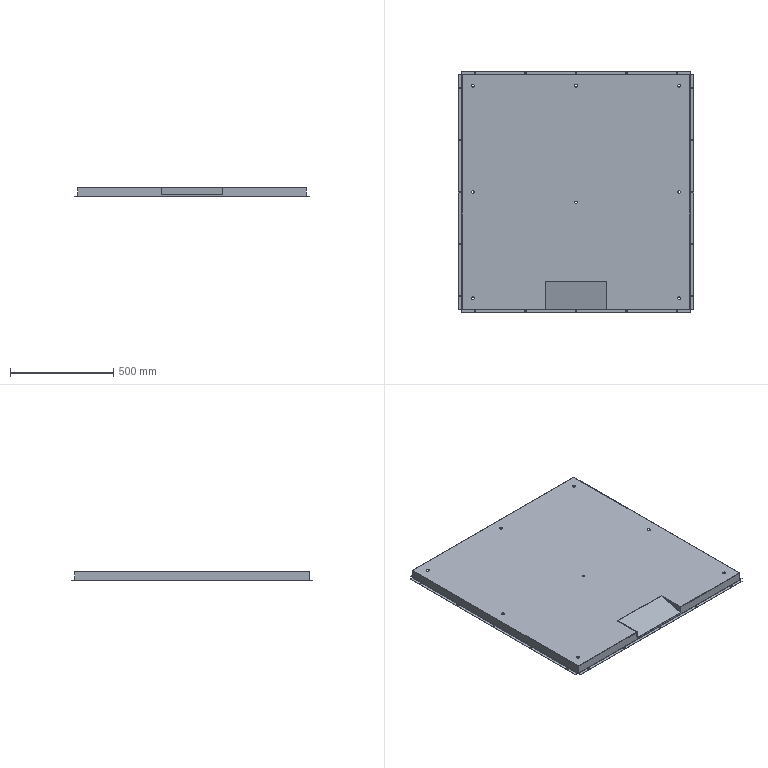Part | 2 solids | 206 faces | box 1140 x 1170 x 44 mm | volume 1514634 mm3 | plane 106 | cylinder 88 | spline 12 | commonest cylinder face diameters 7 x50 14 x14 1 x9 3 x9 0.4 x2 2.4 x2